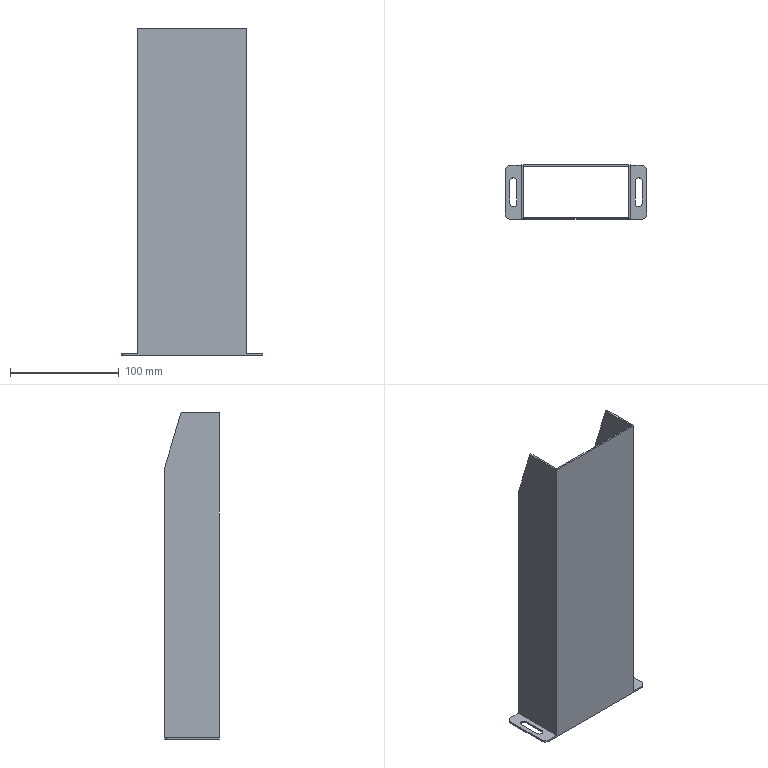Part | SolidWorks | features ICE 4, Cut 1, Fillet 1, MirrorPattern 1, Shell 1 | 1 solid | 29 faces | box 130 x 50 x 300 mm | volume 125628 mm3 | plane 21 | cylinder 8 | commonest cylinder face diameters 6.5 x4 10 x4
STEP:
#1=CARTESIAN_POINT('',(48.5,25.,250.));
#2=VERTEX_POINT('',#1);
#3=CARTESIAN_POINT('',(50.,25.,250.));
#4=VERTEX_POINT('',#3);
#5=CARTESIAN_POINT('',(-65.,25.,250.));
#6=DIRECTION('',(1.,0.,0.));
#7=VECTOR('',#6,1000.);
#8=LINE('',#5,#7);
#9=EDGE_CURVE('',#2,#4,#8,.T.);
#10=ORIENTED_EDGE('',*,*,#9,.F.);
#11=CARTESIAN_POINT('',(48.5,10.,300.));
#12=VERTEX_POINT('',#11);
#13=CARTESIAN_POINT('',(48.5,11.239,295.872));
#14=DIRECTION('',(0.,-0.2873,0.9578));
#15=VECTOR('',#14,1000.);
#16=LINE('',#13,#15);
#17=EDGE_CURVE('',#2,#12,#16,.T.);
#18=ORIENTED_EDGE('',*,*,#17,.T.);
#19=CARTESIAN_POINT('',(50.,10.,300.));
#20=VERTEX_POINT('',#19);
#21=CARTESIAN_POINT('',(-65.,10.,300.));
#22=DIRECTION('',(1.,0.,0.));
#23=VECTOR('',#22,1000.);
#24=LINE('',#21,#23);
#25=EDGE_CURVE('',#12,#20,#24,.T.);
#26=ORIENTED_EDGE('',*,*,#25,.T.);
#27=CARTESIAN_POINT('',(50.,10.,300.));
#28=DIRECTION('',(0.,0.2873,-0.9578));
#29=VECTOR('',#28,1000.);
#30=LINE('',#27,#29);
#31=EDGE_CURVE('',#20,#4,#30,.T.);
#32=ORIENTED_EDGE('',*,*,#31,.T.);
#33=EDGE_LOOP('',(#10,#18,#26,#32));
#34=FACE_OUTER_BOUND('',#33,.T.);
#35=CARTESIAN_POINT('',(-65.,10.,300.));
#36=DIRECTION('',(0.,-0.9578,-0.2873));
#37=DIRECTION('',(0.,0.2873,-0.9578));
#38=AXIS2_PLACEMENT_3D('',#35,#36,#37);
#39=PLANE('',#38);
#40=ADVANCED_FACE('',(#34),#39,.F.);
#41=CARTESIAN_POINT('',(65.,20.,0.));
#42=VERTEX_POINT('',#41);
#43=CARTESIAN_POINT('',(65.,-20.,0.));
#44=VERTEX_POINT('',#43);
#45=CARTESIAN_POINT('',(65.,-25.,0.));
#46=DIRECTION('',(0.,-1.,0.));
#47=VECTOR('',#46,1000.);
#48=LINE('',#45,#47);
#49=EDGE_CURVE('',#42,#44,#48,.T.);
#50=ORIENTED_EDGE('',*,*,#49,.T.);
#51=CARTESIAN_POINT('',(60.,-25.,0.));
#52=VERTEX_POINT('',#51);
#53=CARTESIAN_POINT('',(60.,-20.,0.));
#54=DIRECTION('',(0.,0.,-1.));
#55=DIRECTION('',(1.,0.,0.));
#56=AXIS2_PLACEMENT_3D('',#53,#54,#55);
#57=CIRCLE('',#56,5.);
#58=EDGE_CURVE('',#44,#52,#57,.T.);
#59=ORIENTED_EDGE('',*,*,#58,.T.);
#60=CARTESIAN_POINT('',(-60.,-25.,0.));
#61=VERTEX_POINT('',#60);
#62=CARTESIAN_POINT('',(-50.,-25.,0.));
#63=DIRECTION('',(1.,0.,0.));
#64=VECTOR('',#63,1000.);
#65=LINE('',#62,#64);
#66=EDGE_CURVE('',#61,#52,#65,.T.);
#67=ORIENTED_EDGE('',*,*,#66,.F.);
#68=CARTESIAN_POINT('',(-65.,-20.,0.));
#69=VERTEX_POINT('',#68);
#70=CARTESIAN_POINT('',(-60.,-20.,0.));
#71=DIRECTION('',(0.,0.,-1.));
#72=DIRECTION('',(1.,0.,0.));
#73=AXIS2_PLACEMENT_3D('',#70,#71,#72);
#74=CIRCLE('',#73,5.);
#75=EDGE_CURVE('',#61,#69,#74,.T.);
#76=ORIENTED_EDGE('',*,*,#75,.T.);
#77=CARTESIAN_POINT('',(-65.,20.,0.));
#78=VERTEX_POINT('',#77);
#79=CARTESIAN_POINT('',(-65.,-25.,0.));
#80=DIRECTION('',(0.,1.,0.));
#81=VECTOR('',#80,1000.);
#82=LINE('',#79,#81);
#83=EDGE_CURVE('',#69,#78,#82,.T.);
#84=ORIENTED_EDGE('',*,*,#83,.T.);
#85=CARTESIAN_POINT('',(-60.,25.,0.));
#86=VERTEX_POINT('',#85);
#87=CARTESIAN_POINT('',(-60.,20.,0.));
#88=DIRECTION('',(0.,0.,-1.));
#89=DIRECTION('',(1.,0.,0.));
#90=AXIS2_PLACEMENT_3D('',#87,#88,#89);
#91=CIRCLE('',#90,5.);
#92=EDGE_CURVE('',#78,#86,#91,.T.);
#93=ORIENTED_EDGE('',*,*,#92,.T.);
#94=CARTESIAN_POINT('',(60.,25.,0.));
#95=VERTEX_POINT('',#94);
#96=CARTESIAN_POINT('',(-50.,25.,0.));
#97=DIRECTION('',(-1.,0.,0.));
#98=VECTOR('',#97,1000.);
#99=LINE('',#96,#98);
#100=EDGE_CURVE('',#95,#86,#99,.T.);
#101=ORIENTED_EDGE('',*,*,#100,.F.);
#102=CARTESIAN_POINT('',(60.,20.,0.));
#103=DIRECTION('',(0.,0.,-1.));
#104=DIRECTION('',(1.,0.,0.));
#105=AXIS2_PLACEMENT_3D('',#102,#103,#104);
#106=CIRCLE('',#105,5.);
#107=EDGE_CURVE('',#95,#42,#106,.T.);
#108=ORIENTED_EDGE('',*,*,#107,.T.);
#109=EDGE_LOOP('',(#50,#59,#67,#76,#84,#93,#101,#108));
#110=FACE_OUTER_BOUND('',#109,.T.);
#111=CARTESIAN_POINT('',(-48.5,-23.5,0.));
#112=VERTEX_POINT('',#111);
#113=CARTESIAN_POINT('',(48.5,-23.5,0.));
#114=VERTEX_POINT('',#113);
#115=CARTESIAN_POINT('',(-50.,-23.5,0.));
#116=DIRECTION('',(1.,0.,0.));
#117=VECTOR('',#116,1000.);
#118=LINE('',#115,#117);
#119=EDGE_CURVE('',#112,#114,#118,.T.);
#120=ORIENTED_EDGE('',*,*,#119,.T.);
#121=CARTESIAN_POINT('',(48.5,23.5,0.));
#122=VERTEX_POINT('',#121);
#123=CARTESIAN_POINT('',(48.5,25.,0.));
#124=DIRECTION('',(0.,1.,0.));
#125=VECTOR('',#124,1000.);
#126=LINE('',#123,#125);
#127=EDGE_CURVE('',#114,#122,#126,.T.);
#128=ORIENTED_EDGE('',*,*,#127,.T.);
#129=CARTESIAN_POINT('',(-48.5,23.5,0.));
#130=VERTEX_POINT('',#129);
#131=CARTESIAN_POINT('',(-50.,23.5,0.));
#132=DIRECTION('',(-1.,0.,0.));
#133=VECTOR('',#132,1000.);
#134=LINE('',#131,#133);
#135=EDGE_CURVE('',#122,#130,#134,.T.);
#136=ORIENTED_EDGE('',*,*,#135,.T.);
#137=CARTESIAN_POINT('',(-48.5,25.,0.));
#138=DIRECTION('',(0.,-1.,0.));
#139=VECTOR('',#138,1000.);
#140=LINE('',#137,#139);
#141=EDGE_CURVE('',#130,#112,#140,.T.);
#142=ORIENTED_EDGE('',*,*,#141,.T.);
#143=EDGE_LOOP('',(#120,#128,#136,#142));
#144=FACE_BOUND('',#143,.T.);
#145=CARTESIAN_POINT('',(-60.75,10.,0.));
#146=VERTEX_POINT('',#145);
#147=CARTESIAN_POINT('',(-60.75,-10.,0.));
#148=VERTEX_POINT('',#147);
#149=CARTESIAN_POINT('',(-60.75,-10.,0.));
#150=DIRECTION('',(0.,-1.,0.));
#151=VECTOR('',#150,1000.);
#152=LINE('',#149,#151);
#153=EDGE_CURVE('',#146,#148,#152,.T.);
#154=ORIENTED_EDGE('',*,*,#153,.T.);
#155=CARTESIAN_POINT('',(-54.25,-10.,0.));
#156=VERTEX_POINT('',#155);
#157=CARTESIAN_POINT('',(-57.5,-10.,0.));
#158=DIRECTION('',(0.,0.,1.));
#159=DIRECTION('',(1.,0.,0.));
#160=AXIS2_PLACEMENT_3D('',#157,#158,#159);
#161=CIRCLE('',#160,3.25);
#162=EDGE_CURVE('',#148,#156,#161,.T.);
#163=ORIENTED_EDGE('',*,*,#162,.T.);
#164=CARTESIAN_POINT('',(-54.25,10.,0.));
#165=VERTEX_POINT('',#164);
#166=CARTESIAN_POINT('',(-54.25,-10.,0.));
#167=DIRECTION('',(0.,1.,0.));
#168=VECTOR('',#167,1000.);
#169=LINE('',#166,#168);
#170=EDGE_CURVE('',#156,#165,#169,.T.);
#171=ORIENTED_EDGE('',*,*,#170,.T.);
#172=CARTESIAN_POINT('',(-57.5,10.,0.));
#173=DIRECTION('',(0.,0.,1.));
#174=DIRECTION('',(1.,0.,0.));
#175=AXIS2_PLACEMENT_3D('',#172,#173,#174);
#176=CIRCLE('',#175,3.25);
#177=EDGE_CURVE('',#165,#146,#176,.T.);
#178=ORIENTED_EDGE('',*,*,#177,.T.);
#179=EDGE_LOOP('',(#154,#163,#171,#178));
#180=FACE_BOUND('',#179,.T.);
#181=CARTESIAN_POINT('',(60.75,-10.,0.));
#182=VERTEX_POINT('',#181);
#183=CARTESIAN_POINT('',(54.25,-10.,0.));
#184=VERTEX_POINT('',#183);
#185=CARTESIAN_POINT('',(57.5,-10.,0.));
#186=DIRECTION('',(0.,0.,-1.));
#187=DIRECTION('',(-1.,0.,0.));
#188=AXIS2_PLACEMENT_3D('',#185,#186,#187);
#189=CIRCLE('',#188,3.25);
#190=EDGE_CURVE('',#182,#184,#189,.T.);
#191=ORIENTED_EDGE('',*,*,#190,.F.);
#192=CARTESIAN_POINT('',(60.75,10.,0.));
#193=VERTEX_POINT('',#192);
#194=CARTESIAN_POINT('',(60.75,-10.,0.));
#195=DIRECTION('',(0.,-1.,0.));
#196=VECTOR('',#195,1000.);
#197=LINE('',#194,#196);
#198=EDGE_CURVE('',#193,#182,#197,.T.);
#199=ORIENTED_EDGE('',*,*,#198,.F.);
#200=CARTESIAN_POINT('',(54.25,10.,0.));
#201=VERTEX_POINT('',#200);
#202=CARTESIAN_POINT('',(57.5,10.,0.));
#203=DIRECTION('',(0.,0.,-1.));
#204=DIRECTION('',(-1.,0.,0.));
#205=AXIS2_PLACEMENT_3D('',#202,#203,#204);
#206=CIRCLE('',#205,3.25);
#207=EDGE_CURVE('',#201,#193,#206,.T.);
#208=ORIENTED_EDGE('',*,*,#207,.F.);
#209=CARTESIAN_POINT('',(54.25,-10.,0.));
#210=DIRECTION('',(0.,1.,0.));
#211=VECTOR('',#210,1000.);
#212=LINE('',#209,#211);
#213=EDGE_CURVE('',#184,#201,#212,.T.);
#214=ORIENTED_EDGE('',*,*,#213,.F.);
#215=EDGE_LOOP('',(#191,#199,#208,#214));
#216=FACE_BOUND('',#215,.T.);
#217=CARTESIAN_POINT('',(0.,0.,0.));
#218=DIRECTION('',(0.,0.,1.));
#219=DIRECTION('',(1.,0.,0.));
#220=AXIS2_PLACEMENT_3D('',#217,#218,#219);
#221=PLANE('',#220);
#222=ADVANCED_FACE('',(#110,#144,#180,#216),#221,.F.);
#223=CARTESIAN_POINT('',(60.,-25.,1.5));
#224=VERTEX_POINT('',#223);
#225=CARTESIAN_POINT('',(50.,-25.,1.5));
#226=VERTEX_POINT('',#225);
#227=CARTESIAN_POINT('',(50.,-25.,1.5));
#228=DIRECTION('',(-1.,0.,0.));
#229=VECTOR('',#228,1000.);
#230=LINE('',#227,#229);
#231=EDGE_CURVE('',#224,#226,#230,.T.);
#232=ORIENTED_EDGE('',*,*,#231,.F.);
#233=CARTESIAN_POINT('',(65.,-20.,1.5));
#234=VERTEX_POINT('',#233);
#235=CARTESIAN_POINT('',(60.,-20.,1.5));
#236=DIRECTION('',(0.,0.,1.));
#237=DIRECTION('',(-1.,0.,0.));
#238=AXIS2_PLACEMENT_3D('',#235,#236,#237);
#239=CIRCLE('',#238,5.);
#240=EDGE_CURVE('',#224,#234,#239,.T.);
#241=ORIENTED_EDGE('',*,*,#240,.T.);
#242=CARTESIAN_POINT('',(65.,20.,1.5));
#243=VERTEX_POINT('',#242);
#244=CARTESIAN_POINT('',(65.,-25.,1.5));
#245=DIRECTION('',(0.,-1.,0.));
#246=VECTOR('',#245,1000.);
#247=LINE('',#244,#246);
#248=EDGE_CURVE('',#243,#234,#247,.T.);
#249=ORIENTED_EDGE('',*,*,#248,.F.);
#250=CARTESIAN_POINT('',(60.,25.,1.5));
#251=VERTEX_POINT('',#250);
#252=CARTESIAN_POINT('',(60.,20.,1.5));
#253=DIRECTION('',(0.,0.,1.));
#254=DIRECTION('',(-1.,0.,0.));
#255=AXIS2_PLACEMENT_3D('',#252,#253,#254);
#256=CIRCLE('',#255,5.);
#257=EDGE_CURVE('',#243,#251,#256,.T.);
#258=ORIENTED_EDGE('',*,*,#257,.T.);
#259=CARTESIAN_POINT('',(50.,25.,1.5));
#260=VERTEX_POINT('',#259);
#261=CARTESIAN_POINT('',(50.,25.,1.5));
#262=DIRECTION('',(1.,0.,0.));
#263=VECTOR('',#262,1000.);
#264=LINE('',#261,#263);
#265=EDGE_CURVE('',#260,#251,#264,.T.);
#266=ORIENTED_EDGE('',*,*,#265,.F.);
#267=CARTESIAN_POINT('',(50.,-25.,1.5));
#268=DIRECTION('',(0.,1.,0.));
#269=VECTOR('',#268,1000.);
#270=LINE('',#267,#269);
#271=EDGE_CURVE('',#226,#260,#270,.T.);
#272=ORIENTED_EDGE('',*,*,#271,.F.);
#273=EDGE_LOOP('',(#232,#241,#249,#258,#266,#272));
#274=FACE_OUTER_BOUND('',#273,.T.);
#275=CARTESIAN_POINT('',(60.75,-10.,1.5));
#276=VERTEX_POINT('',#275);
#277=CARTESIAN_POINT('',(54.25,-10.,1.5));
#278=VERTEX_POINT('',#277);
#279=CARTESIAN_POINT('',(57.5,-10.,1.5));
#280=DIRECTION('',(0.,0.,-1.));
#281=DIRECTION('',(-1.,0.,0.));
#282=AXIS2_PLACEMENT_3D('',#279,#280,#281);
#283=CIRCLE('',#282,3.25);
#284=EDGE_CURVE('',#276,#278,#283,.T.);
#285=ORIENTED_EDGE('',*,*,#284,.T.);
#286=CARTESIAN_POINT('',(54.25,10.,1.5));
#287=VERTEX_POINT('',#286);
#288=CARTESIAN_POINT('',(54.25,-10.,1.5));
#289=DIRECTION('',(0.,1.,0.));
#290=VECTOR('',#289,1000.);
#291=LINE('',#288,#290);
#292=EDGE_CURVE('',#278,#287,#291,.T.);
#293=ORIENTED_EDGE('',*,*,#292,.T.);
#294=CARTESIAN_POINT('',(60.75,10.,1.5));
#295=VERTEX_POINT('',#294);
#296=CARTESIAN_POINT('',(57.5,10.,1.5));
#297=DIRECTION('',(0.,0.,-1.));
#298=DIRECTION('',(-1.,0.,0.));
#299=AXIS2_PLACEMENT_3D('',#296,#297,#298);
#300=CIRCLE('',#299,3.25);
#301=EDGE_CURVE('',#287,#295,#300,.T.);
#302=ORIENTED_EDGE('',*,*,#301,.T.);
#303=CARTESIAN_POINT('',(60.75,-10.,1.5));
#304=DIRECTION('',(0.,-1.,0.));
#305=VECTOR('',#304,1000.);
#306=LINE('',#303,#305);
#307=EDGE_CURVE('',#295,#276,#306,.T.);
#308=ORIENTED_EDGE('',*,*,#307,.T.);
#309=EDGE_LOOP('',(#285,#293,#302,#308));
#310=FACE_BOUND('',#309,.T.);
#311=CARTESIAN_POINT('',(0.,0.,1.5));
#312=DIRECTION('',(0.,0.,-1.));
#313=DIRECTION('',(-1.,0.,0.));
#314=AXIS2_PLACEMENT_3D('',#311,#312,#313);
#315=PLANE('',#314);
#316=ADVANCED_FACE('',(#274,#310),#315,.F.);
#317=CARTESIAN_POINT('',(50.,25.,300.));
#318=DIRECTION('',(0.,0.,-1.));
#319=VECTOR('',#318,1000.);
#320=LINE('',#317,#319);
#321=EDGE_CURVE('',#4,#260,#320,.T.);
#322=ORIENTED_EDGE('',*,*,#321,.F.);
#323=ORIENTED_EDGE('',*,*,#31,.F.);
#324=CARTESIAN_POINT('',(50.,-25.,300.));
#325=VERTEX_POINT('',#324);
#326=CARTESIAN_POINT('',(50.,25.,300.));
#327=DIRECTION('',(0.,1.,0.));
#328=VECTOR('',#327,1000.);
#329=LINE('',#326,#328);
#330=EDGE_CURVE('',#325,#20,#329,.T.);
#331=ORIENTED_EDGE('',*,*,#330,.F.);
#332=CARTESIAN_POINT('',(50.,-25.,300.));
#333=DIRECTION('',(0.,0.,-1.));
#334=VECTOR('',#333,1000.);
#335=LINE('',#332,#334);
#336=EDGE_CURVE('',#325,#226,#335,.T.);
#337=ORIENTED_EDGE('',*,*,#336,.T.);
#338=ORIENTED_EDGE('',*,*,#271,.T.);
#339=EDGE_LOOP('',(#322,#323,#331,#337,#338));
#340=FACE_OUTER_BOUND('',#339,.T.);
#341=CARTESIAN_POINT('',(50.,25.,300.));
#342=DIRECTION('',(-1.,0.,0.));
#343=DIRECTION('',(0.,-1.,0.));
#344=AXIS2_PLACEMENT_3D('',#341,#342,#343);
#345=PLANE('',#344);
#346=ADVANCED_FACE('',(#340),#345,.F.);
#347=ORIENTED_EDGE('',*,*,#265,.T.);
#348=CARTESIAN_POINT('',(60.,25.,0.));
#349=DIRECTION('',(0.,0.,-1.));
#350=VECTOR('',#349,1000.);
#351=LINE('',#348,#350);
#352=EDGE_CURVE('',#251,#95,#351,.T.);
#353=ORIENTED_EDGE('',*,*,#352,.T.);
#354=ORIENTED_EDGE('',*,*,#100,.T.);
#355=CARTESIAN_POINT('',(-60.,25.,1.5));
#356=VERTEX_POINT('',#355);
#357=CARTESIAN_POINT('',(-60.,25.,1.5));
#358=DIRECTION('',(0.,0.,1.));
#359=VECTOR('',#358,1000.);
#360=LINE('',#357,#359);
#361=EDGE_CURVE('',#86,#356,#360,.T.);
#362=ORIENTED_EDGE('',*,*,#361,.T.);
#363=CARTESIAN_POINT('',(-50.,25.,1.5));
#364=VERTEX_POINT('',#363);
#365=CARTESIAN_POINT('',(-65.,25.,1.5));
#366=DIRECTION('',(1.,0.,0.));
#367=VECTOR('',#366,1000.);
#368=LINE('',#365,#367);
#369=EDGE_CURVE('',#356,#364,#368,.T.);
#370=ORIENTED_EDGE('',*,*,#369,.T.);
#371=CARTESIAN_POINT('',(-50.,25.,250.));
#372=VERTEX_POINT('',#371);
#373=CARTESIAN_POINT('',(-50.,25.,300.));
#374=DIRECTION('',(0.,0.,-1.));
#375=VECTOR('',#374,1000.);
#376=LINE('',#373,#375);
#377=EDGE_CURVE('',#372,#364,#376,.T.);
#378=ORIENTED_EDGE('',*,*,#377,.F.);
#379=CARTESIAN_POINT('',(-48.5,25.,250.));
#380=VERTEX_POINT('',#379);
#381=CARTESIAN_POINT('',(-65.,25.,250.));
#382=DIRECTION('',(1.,0.,0.));
#383=VECTOR('',#382,1000.);
#384=LINE('',#381,#383);
#385=EDGE_CURVE('',#372,#380,#384,.T.);
#386=ORIENTED_EDGE('',*,*,#385,.T.);
#387=CARTESIAN_POINT('',(-48.5,25.,250.));
#388=DIRECTION('',(-1.,0.,0.));
#389=VECTOR('',#388,1000.);
#390=LINE('',#387,#389);
#391=EDGE_CURVE('',#2,#380,#390,.T.);
#392=ORIENTED_EDGE('',*,*,#391,.F.);
#393=ORIENTED_EDGE('',*,*,#9,.T.);
#394=ORIENTED_EDGE('',*,*,#321,.T.);
#395=EDGE_LOOP('',(#347,#353,#354,#362,#370,#378,#386,#392,#393,#394));
#396=FACE_OUTER_BOUND('',#395,.T.);
#397=CARTESIAN_POINT('',(-50.,25.,300.));
#398=DIRECTION('',(0.,-1.,0.));
#399=DIRECTION('',(0.,0.,-1.));
#400=AXIS2_PLACEMENT_3D('',#397,#398,#399);
#401=PLANE('',#400);
#402=ADVANCED_FACE('',(#396),#401,.F.);
#403=CARTESIAN_POINT('',(-50.,10.,300.));
#404=VERTEX_POINT('',#403);
#405=CARTESIAN_POINT('',(-50.,-25.,300.));
#406=VERTEX_POINT('',#405);
#407=CARTESIAN_POINT('',(-50.,25.,300.));
#408=DIRECTION('',(0.,-1.,0.));
#409=VECTOR('',#408,1000.);
#410=LINE('',#407,#409);
#411=EDGE_CURVE('',#404,#406,#410,.T.);
#412=ORIENTED_EDGE('',*,*,#411,.F.);
#413=CARTESIAN_POINT('',(-50.,11.239,295.872));
#414=DIRECTION('',(0.,0.2873,-0.9578));
#415=VECTOR('',#414,1000.);
#416=LINE('',#413,#415);
#417=EDGE_CURVE('',#404,#372,#416,.T.);
#418=ORIENTED_EDGE('',*,*,#417,.T.);
#419=ORIENTED_EDGE('',*,*,#377,.T.);
#420=CARTESIAN_POINT('',(-50.,-25.,1.5));
#421=VERTEX_POINT('',#420);
#422=CARTESIAN_POINT('',(-50.,-25.,1.5));
#423=DIRECTION('',(0.,-1.,0.));
#424=VECTOR('',#423,1000.);
#425=LINE('',#422,#424);
#426=EDGE_CURVE('',#364,#421,#425,.T.);
#427=ORIENTED_EDGE('',*,*,#426,.T.);
#428=CARTESIAN_POINT('',(-50.,-25.,300.));
#429=DIRECTION('',(0.,0.,-1.));
#430=VECTOR('',#429,1000.);
#431=LINE('',#428,#430);
#432=EDGE_CURVE('',#406,#421,#431,.T.);
#433=ORIENTED_EDGE('',*,*,#432,.F.);
#434=EDGE_LOOP('',(#412,#418,#419,#427,#433));
#435=FACE_OUTER_BOUND('',#434,.T.);
#436=CARTESIAN_POINT('',(-50.,25.,300.));
#437=DIRECTION('',(1.,0.,0.));
#438=DIRECTION('',(0.,1.,0.));
#439=AXIS2_PLACEMENT_3D('',#436,#437,#438);
#440=PLANE('',#439);
#441=ADVANCED_FACE('',(#435),#440,.F.);
#442=ORIENTED_EDGE('',*,*,#66,.T.);
#443=CARTESIAN_POINT('',(60.,-25.,1.5));
#444=DIRECTION('',(0.,0.,1.));
#445=VECTOR('',#444,1000.);
#446=LINE('',#443,#445);
#447=EDGE_CURVE('',#52,#224,#446,.T.);
#448=ORIENTED_EDGE('',*,*,#447,.T.);
#449=ORIENTED_EDGE('',*,*,#231,.T.);
#450=ORIENTED_EDGE('',*,*,#336,.F.);
#451=CARTESIAN_POINT('',(-50.,-25.,300.));
#452=DIRECTION('',(1.,0.,0.));
#453=VECTOR('',#452,1000.);
#454=LINE('',#451,#453);
#455=EDGE_CURVE('',#406,#325,#454,.T.);
#456=ORIENTED_EDGE('',*,*,#455,.F.);
#457=ORIENTED_EDGE('',*,*,#432,.T.);
#458=CARTESIAN_POINT('',(-60.,-25.,1.5));
#459=VERTEX_POINT('',#458);
#460=CARTESIAN_POINT('',(-65.,-25.,1.5));
#461=DIRECTION('',(-1.,0.,0.));
#462=VECTOR('',#461,1000.);
#463=LINE('',#460,#462);
#464=EDGE_CURVE('',#421,#459,#463,.T.);
#465=ORIENTED_EDGE('',*,*,#464,.T.);
#466=CARTESIAN_POINT('',(-60.,-25.,0.));
#467=DIRECTION('',(0.,0.,-1.));
#468=VECTOR('',#467,1000.);
#469=LINE('',#466,#468);
#470=EDGE_CURVE('',#459,#61,#469,.T.);
#471=ORIENTED_EDGE('',*,*,#470,.T.);
#472=EDGE_LOOP('',(#442,#448,#449,#450,#456,#457,#465,#471));
#473=FACE_OUTER_BOUND('',#472,.T.);
#474=CARTESIAN_POINT('',(-50.,-25.,300.));
#475=DIRECTION('',(0.,1.,0.));
#476=DIRECTION('',(0.,0.,1.));
#477=AXIS2_PLACEMENT_3D('',#474,#475,#476);
#478=PLANE('',#477);
#479=ADVANCED_FACE('',(#473),#478,.F.);
#480=CARTESIAN_POINT('',(-48.5,10.,300.));
#481=VERTEX_POINT('',#480);
#482=CARTESIAN_POINT('',(-65.,10.,300.));
#483=DIRECTION('',(1.,0.,0.));
#484=VECTOR('',#483,1000.);
#485=LINE('',#482,#484);
#486=EDGE_CURVE('',#404,#481,#485,.T.);
#487=ORIENTED_EDGE('',*,*,#486,.F.);
#488=ORIENTED_EDGE('',*,*,#411,.T.);
#489=ORIENTED_EDGE('',*,*,#455,.T.);
#490=ORIENTED_EDGE('',*,*,#330,.T.);
#491=ORIENTED_EDGE('',*,*,#25,.F.);
#492=CARTESIAN_POINT('',(48.5,-23.5,300.));
#493=VERTEX_POINT('',#492);
#494=CARTESIAN_POINT('',(48.5,25.,300.));
#495=DIRECTION('',(0.,1.,0.));
#496=VECTOR('',#495,1000.);
#497=LINE('',#494,#496);
#498=EDGE_CURVE('',#493,#12,#497,.T.);
#499=ORIENTED_EDGE('',*,*,#498,.F.);
#500=CARTESIAN_POINT('',(-48.5,-23.5,300.));
#501=VERTEX_POINT('',#500);
#502=CARTESIAN_POINT('',(-50.,-23.5,300.));
#503=DIRECTION('',(1.,0.,0.));
#504=VECTOR('',#503,1000.);
#505=LINE('',#502,#504);
#506=EDGE_CURVE('',#501,#493,#505,.T.);
#507=ORIENTED_EDGE('',*,*,#506,.F.);
#508=CARTESIAN_POINT('',(-48.5,25.,300.));
#509=DIRECTION('',(0.,-1.,0.));
#510=VECTOR('',#509,1000.);
#511=LINE('',#508,#510);
#512=EDGE_CURVE('',#481,#501,#511,.T.);
#513=ORIENTED_EDGE('',*,*,#512,.F.);
#514=EDGE_LOOP('',(#487,#488,#489,#490,#491,#499,#507,#513));
#515=FACE_OUTER_BOUND('',#514,.T.);
#516=CARTESIAN_POINT('',(0.,0.,300.));
#517=DIRECTION('',(0.,0.,1.));
#518=DIRECTION('',(1.,0.,0.));
#519=AXIS2_PLACEMENT_3D('',#516,#517,#518);
#520=PLANE('',#519);
#521=ADVANCED_FACE('',(#515),#520,.T.);
#522=ORIENTED_EDGE('',*,*,#17,.F.);
#523=CARTESIAN_POINT('',(48.5,23.5,250.));
#524=VERTEX_POINT('',#523);
#525=CARTESIAN_POINT('',(48.5,-25.001,250.));
#526=DIRECTION('',(0.,1.,0.));
#527=VECTOR('',#526,1000.);
#528=LINE('',#525,#527);
#529=EDGE_CURVE('',#524,#2,#528,.T.);
#530=ORIENTED_EDGE('',*,*,#529,.F.);
#531=CARTESIAN_POINT('',(48.5,23.5,300.));
#532=DIRECTION('',(0.,0.,-1.));
#533=VECTOR('',#532,1000.);
#534=LINE('',#531,#533);
#535=EDGE_CURVE('',#524,#122,#534,.T.);
#536=ORIENTED_EDGE('',*,*,#535,.T.);
#537=ORIENTED_EDGE('',*,*,#127,.F.);
#538=CARTESIAN_POINT('',(48.5,-23.5,300.));
#539=DIRECTION('',(0.,0.,-1.));
#540=VECTOR('',#539,1000.);
#541=LINE('',#538,#540);
#542=EDGE_CURVE('',#493,#114,#541,.T.);
#543=ORIENTED_EDGE('',*,*,#542,.F.);
#544=ORIENTED_EDGE('',*,*,#498,.T.);
#545=EDGE_LOOP('',(#522,#530,#536,#537,#543,#544));
#546=FACE_OUTER_BOUND('',#545,.T.);
#547=CARTESIAN_POINT('',(48.5,25.,300.));
#548=DIRECTION('',(-1.,0.,0.));
#549=DIRECTION('',(0.,-1.,0.));
#550=AXIS2_PLACEMENT_3D('',#547,#548,#549);
#551=PLANE('',#550);
#552=ADVANCED_FACE('',(#546),#551,.T.);
#553=CARTESIAN_POINT('',(-48.5,23.5,250.));
#554=VERTEX_POINT('',#553);
#555=CARTESIAN_POINT('',(-48.5,23.5,250.));
#556=DIRECTION('',(-1.,0.,0.));
#557=VECTOR('',#556,1000.);
#558=LINE('',#555,#557);
#559=EDGE_CURVE('',#524,#554,#558,.T.);
#560=ORIENTED_EDGE('',*,*,#559,.T.);
#561=CARTESIAN_POINT('',(-48.5,23.5,300.));
#562=DIRECTION('',(0.,0.,-1.));
#563=VECTOR('',#562,1000.);
#564=LINE('',#561,#563);
#565=EDGE_CURVE('',#554,#130,#564,.T.);
#566=ORIENTED_EDGE('',*,*,#565,.T.);
#567=ORIENTED_EDGE('',*,*,#135,.F.);
#568=ORIENTED_EDGE('',*,*,#535,.F.);
#569=EDGE_LOOP('',(#560,#566,#567,#568));
#570=FACE_OUTER_BOUND('',#569,.T.);
#571=CARTESIAN_POINT('',(-50.,23.5,300.));
#572=DIRECTION('',(0.,-1.,0.));
#573=DIRECTION('',(0.,0.,-1.));
#574=AXIS2_PLACEMENT_3D('',#571,#572,#573);
#575=PLANE('',#574);
#576=ADVANCED_FACE('',(#570),#575,.T.);
#577=CARTESIAN_POINT('',(-48.5,11.239,295.872));
#578=DIRECTION('',(0.,0.2873,-0.9578));
#579=VECTOR('',#578,1000.);
#580=LINE('',#577,#579);
#581=EDGE_CURVE('',#481,#380,#580,.T.);
#582=ORIENTED_EDGE('',*,*,#581,.F.);
#583=ORIENTED_EDGE('',*,*,#512,.T.);
#584=CARTESIAN_POINT('',(-48.5,-23.5,300.));
#585=DIRECTION('',(0.,0.,-1.));
#586=VECTOR('',#585,1000.);
#587=LINE('',#584,#586);
#588=EDGE_CURVE('',#501,#112,#587,.T.);
#589=ORIENTED_EDGE('',*,*,#588,.T.);
#590=ORIENTED_EDGE('',*,*,#141,.F.);
#591=ORIENTED_EDGE('',*,*,#565,.F.);
#592=CARTESIAN_POINT('',(-48.5,-25.001,250.));
#593=DIRECTION('',(0.,1.,0.));
#594=VECTOR('',#593,1000.);
#595=LINE('',#592,#594);
#596=EDGE_CURVE('',#554,#380,#595,.T.);
#597=ORIENTED_EDGE('',*,*,#596,.T.);
#598=EDGE_LOOP('',(#582,#583,#589,#590,#591,#597));
#599=FACE_OUTER_BOUND('',#598,.T.);
#600=CARTESIAN_POINT('',(-48.5,25.,300.));
#601=DIRECTION('',(1.,0.,0.));
#602=DIRECTION('',(0.,1.,0.));
#603=AXIS2_PLACEMENT_3D('',#600,#601,#602);
#604=PLANE('',#603);
#605=ADVANCED_FACE('',(#599),#604,.T.);
#606=ORIENTED_EDGE('',*,*,#119,.F.);
#607=ORIENTED_EDGE('',*,*,#588,.F.);
#608=ORIENTED_EDGE('',*,*,#506,.T.);
#609=ORIENTED_EDGE('',*,*,#542,.T.);
#610=EDGE_LOOP('',(#606,#607,#608,#609));
#611=FACE_OUTER_BOUND('',#610,.T.);
#612=CARTESIAN_POINT('',(-50.,-23.5,300.));
#613=DIRECTION('',(0.,1.,0.));
#614=DIRECTION('',(0.,0.,1.));
#615=AXIS2_PLACEMENT_3D('',#612,#613,#614);
#616=PLANE('',#615);
#617=ADVANCED_FACE('',(#611),#616,.T.);
#618=ORIENTED_EDGE('',*,*,#248,.T.);
#619=CARTESIAN_POINT('',(65.,-20.,0.));
#620=DIRECTION('',(0.,0.,-1.));
#621=VECTOR('',#620,1000.);
#622=LINE('',#619,#621);
#623=EDGE_CURVE('',#234,#44,#622,.T.);
#624=ORIENTED_EDGE('',*,*,#623,.T.);
#625=ORIENTED_EDGE('',*,*,#49,.F.);
#626=CARTESIAN_POINT('',(65.,20.,1.5));
#627=DIRECTION('',(0.,0.,1.));
#628=VECTOR('',#627,1000.);
#629=LINE('',#626,#628);
#630=EDGE_CURVE('',#42,#243,#629,.T.);
#631=ORIENTED_EDGE('',*,*,#630,.T.);
#632=EDGE_LOOP('',(#618,#624,#625,#631));
#633=FACE_OUTER_BOUND('',#632,.T.);
#634=CARTESIAN_POINT('',(65.,-25.,1.5));
#635=DIRECTION('',(1.,0.,0.));
#636=DIRECTION('',(0.,0.,-1.));
#637=AXIS2_PLACEMENT_3D('',#634,#635,#636);
#638=PLANE('',#637);
#639=ADVANCED_FACE('',(#633),#638,.T.);
#640=ORIENTED_EDGE('',*,*,#83,.F.);
#641=CARTESIAN_POINT('',(-65.,-20.,1.5));
#642=VERTEX_POINT('',#641);
#643=CARTESIAN_POINT('',(-65.,-20.,1.5));
#644=DIRECTION('',(0.,0.,1.));
#645=VECTOR('',#644,1000.);
#646=LINE('',#643,#645);
#647=EDGE_CURVE('',#69,#642,#646,.T.);
#648=ORIENTED_EDGE('',*,*,#647,.T.);
#649=CARTESIAN_POINT('',(-65.,20.,1.5));
#650=VERTEX_POINT('',#649);
#651=CARTESIAN_POINT('',(-65.,-25.,1.5));
#652=DIRECTION('',(0.,1.,0.));
#653=VECTOR('',#652,1000.);
#654=LINE('',#651,#653);
#655=EDGE_CURVE('',#642,#650,#654,.T.);
#656=ORIENTED_EDGE('',*,*,#655,.T.);
#657=CARTESIAN_POINT('',(-65.,20.,0.));
#658=DIRECTION('',(0.,0.,-1.));
#659=VECTOR('',#658,1000.);
#660=LINE('',#657,#659);
#661=EDGE_CURVE('',#650,#78,#660,.T.);
#662=ORIENTED_EDGE('',*,*,#661,.T.);
#663=EDGE_LOOP('',(#640,#648,#656,#662));
#664=FACE_OUTER_BOUND('',#663,.T.);
#665=CARTESIAN_POINT('',(-65.,-25.,1.5));
#666=DIRECTION('',(-1.,0.,0.));
#667=DIRECTION('',(0.,0.,1.));
#668=AXIS2_PLACEMENT_3D('',#665,#666,#667);
#669=PLANE('',#668);
#670=ADVANCED_FACE('',(#664),#669,.T.);
#671=CARTESIAN_POINT('',(-54.25,-10.,1.5));
#672=VERTEX_POINT('',#671);
#673=CARTESIAN_POINT('',(-54.25,10.,1.5));
#674=VERTEX_POINT('',#673);
#675=CARTESIAN_POINT('',(-54.25,-10.,1.5));
#676=DIRECTION('',(0.,1.,0.));
#677=VECTOR('',#676,1000.);
#678=LINE('',#675,#677);
#679=EDGE_CURVE('',#672,#674,#678,.T.);
#680=ORIENTED_EDGE('',*,*,#679,.F.);
#681=CARTESIAN_POINT('',(-60.75,-10.,1.5));
#682=VERTEX_POINT('',#681);
#683=CARTESIAN_POINT('',(-57.5,-10.,1.5));
#684=DIRECTION('',(0.,0.,1.));
#685=DIRECTION('',(1.,0.,0.));
#686=AXIS2_PLACEMENT_3D('',#683,#684,#685);
#687=CIRCLE('',#686,3.25);
#688=EDGE_CURVE('',#682,#672,#687,.T.);
#689=ORIENTED_EDGE('',*,*,#688,.F.);
#690=CARTESIAN_POINT('',(-60.75,10.,1.5));
#691=VERTEX_POINT('',#690);
#692=CARTESIAN_POINT('',(-60.75,-10.,1.5));
#693=DIRECTION('',(0.,-1.,0.));
#694=VECTOR('',#693,1000.);
#695=LINE('',#692,#694);
#696=EDGE_CURVE('',#691,#682,#695,.T.);
#697=ORIENTED_EDGE('',*,*,#696,.F.);
#698=CARTESIAN_POINT('',(-57.5,10.,1.5));
#699=DIRECTION('',(0.,0.,1.));
#700=DIRECTION('',(1.,0.,0.));
#701=AXIS2_PLACEMENT_3D('',#698,#699,#700);
#702=CIRCLE('',#701,3.25);
#703=EDGE_CURVE('',#674,#691,#702,.T.);
#704=ORIENTED_EDGE('',*,*,#703,.F.);
#705=EDGE_LOOP('',(#680,#689,#697,#704));
#706=FACE_BOUND('',#705,.T.);
#707=ORIENTED_EDGE('',*,*,#655,.F.);
#708=CARTESIAN_POINT('',(-60.,-20.,1.5));
#709=DIRECTION('',(0.,0.,1.));
#710=DIRECTION('',(-1.,0.,0.));
#711=AXIS2_PLACEMENT_3D('',#708,#709,#710);
#712=CIRCLE('',#711,5.);
#713=EDGE_CURVE('',#642,#459,#712,.T.);
#714=ORIENTED_EDGE('',*,*,#713,.T.);
#715=ORIENTED_EDGE('',*,*,#464,.F.);
#716=ORIENTED_EDGE('',*,*,#426,.F.);
#717=ORIENTED_EDGE('',*,*,#369,.F.);
#718=CARTESIAN_POINT('',(-60.,20.,1.5));
#719=DIRECTION('',(0.,0.,1.));
#720=DIRECTION('',(-1.,0.,0.));
#721=AXIS2_PLACEMENT_3D('',#718,#719,#720);
#722=CIRCLE('',#721,5.);
#723=EDGE_CURVE('',#356,#650,#722,.T.);
#724=ORIENTED_EDGE('',*,*,#723,.T.);
#725=EDGE_LOOP('',(#707,#714,#715,#716,#717,#724));
#726=FACE_OUTER_BOUND('',#725,.T.);
#727=CARTESIAN_POINT('',(0.,0.,1.5));
#728=DIRECTION('',(0.,0.,-1.));
#729=DIRECTION('',(-1.,0.,0.));
#730=AXIS2_PLACEMENT_3D('',#727,#728,#729);
#731=PLANE('',#730);
#732=ADVANCED_FACE('',(#706,#726),#731,.F.);
#733=ORIENTED_EDGE('',*,*,#581,.T.);
#734=ORIENTED_EDGE('',*,*,#385,.F.);
#735=ORIENTED_EDGE('',*,*,#417,.F.);
#736=ORIENTED_EDGE('',*,*,#486,.T.);
#737=EDGE_LOOP('',(#733,#734,#735,#736));
#738=FACE_OUTER_BOUND('',#737,.T.);
#739=CARTESIAN_POINT('',(-65.,10.,300.));
#740=DIRECTION('',(0.,-0.9578,-0.2873));
#741=DIRECTION('',(0.,0.2873,-0.9578));
#742=AXIS2_PLACEMENT_3D('',#739,#740,#741);
#743=PLANE('',#742);
#744=ADVANCED_FACE('',(#738),#743,.F.);
#745=ORIENTED_EDGE('',*,*,#240,.F.);
#746=ORIENTED_EDGE('',*,*,#447,.F.);
#747=ORIENTED_EDGE('',*,*,#58,.F.);
#748=ORIENTED_EDGE('',*,*,#623,.F.);
#749=EDGE_LOOP('',(#745,#746,#747,#748));
#750=FACE_OUTER_BOUND('',#749,.T.);
#751=CARTESIAN_POINT('',(60.,-20.,1.5));
#752=DIRECTION('',(0.,0.,1.));
#753=DIRECTION('',(1.,0.,0.));
#754=AXIS2_PLACEMENT_3D('',#751,#752,#753);
#755=CYLINDRICAL_SURFACE('',#754,5.);
#756=ADVANCED_FACE('',(#750),#755,.T.);
#757=ORIENTED_EDGE('',*,*,#257,.F.);
#758=ORIENTED_EDGE('',*,*,#630,.F.);
#759=ORIENTED_EDGE('',*,*,#107,.F.);
#760=ORIENTED_EDGE('',*,*,#352,.F.);
#761=EDGE_LOOP('',(#757,#758,#759,#760));
#762=FACE_OUTER_BOUND('',#761,.T.);
#763=CARTESIAN_POINT('',(60.,20.,300.));
#764=DIRECTION('',(0.,0.,1.));
#765=DIRECTION('',(1.,0.,0.));
#766=AXIS2_PLACEMENT_3D('',#763,#764,#765);
#767=CYLINDRICAL_SURFACE('',#766,5.);
#768=ADVANCED_FACE('',(#762),#767,.T.);
#769=ORIENTED_EDGE('',*,*,#713,.F.);
#770=ORIENTED_EDGE('',*,*,#647,.F.);
#771=ORIENTED_EDGE('',*,*,#75,.F.);
#772=ORIENTED_EDGE('',*,*,#470,.F.);
#773=EDGE_LOOP('',(#769,#770,#771,#772));
#774=FACE_OUTER_BOUND('',#773,.T.);
#775=CARTESIAN_POINT('',(-60.,-20.,300.));
#776=DIRECTION('',(0.,0.,1.));
#777=DIRECTION('',(1.,0.,0.));
#778=AXIS2_PLACEMENT_3D('',#775,#776,#777);
#779=CYLINDRICAL_SURFACE('',#778,5.);
#780=ADVANCED_FACE('',(#774),#779,.T.);
#781=ORIENTED_EDGE('',*,*,#723,.F.);
#782=ORIENTED_EDGE('',*,*,#361,.F.);
#783=ORIENTED_EDGE('',*,*,#92,.F.);
#784=ORIENTED_EDGE('',*,*,#661,.F.);
#785=EDGE_LOOP('',(#781,#782,#783,#784));
#786=FACE_OUTER_BOUND('',#785,.T.);
#787=CARTESIAN_POINT('',(-60.,20.,1.5));
#788=DIRECTION('',(0.,0.,1.));
#789=DIRECTION('',(1.,0.,0.));
#790=AXIS2_PLACEMENT_3D('',#787,#788,#789);
#791=CYLINDRICAL_SURFACE('',#790,5.);
#792=ADVANCED_FACE('',(#786),#791,.T.);
#793=ORIENTED_EDGE('',*,*,#688,.T.);
#794=CARTESIAN_POINT('',(-54.25,-10.,0.));
#795=DIRECTION('',(0.,0.,1.));
#796=VECTOR('',#795,1000.);
#797=LINE('',#794,#796);
#798=EDGE_CURVE('',#156,#672,#797,.T.);
#799=ORIENTED_EDGE('',*,*,#798,.F.);
#800=ORIENTED_EDGE('',*,*,#162,.F.);
#801=CARTESIAN_POINT('',(-60.75,-10.,0.));
#802=DIRECTION('',(0.,0.,1.));
#803=VECTOR('',#802,1000.);
#804=LINE('',#801,#803);
#805=EDGE_CURVE('',#148,#682,#804,.T.);
#806=ORIENTED_EDGE('',*,*,#805,.T.);
#807=EDGE_LOOP('',(#793,#799,#800,#806));
#808=FACE_OUTER_BOUND('',#807,.T.);
#809=CARTESIAN_POINT('',(-57.5,-10.,0.));
#810=DIRECTION('',(0.,0.,1.));
#811=DIRECTION('',(1.,0.,0.));
#812=AXIS2_PLACEMENT_3D('',#809,#810,#811);
#813=CYLINDRICAL_SURFACE('',#812,3.25);
#814=ADVANCED_FACE('',(#808),#813,.F.);
#815=ORIENTED_EDGE('',*,*,#696,.T.);
#816=ORIENTED_EDGE('',*,*,#805,.F.);
#817=ORIENTED_EDGE('',*,*,#153,.F.);
#818=CARTESIAN_POINT('',(-60.75,10.,0.));
#819=DIRECTION('',(0.,0.,1.));
#820=VECTOR('',#819,1000.);
#821=LINE('',#818,#820);
#822=EDGE_CURVE('',#146,#691,#821,.T.);
#823=ORIENTED_EDGE('',*,*,#822,.T.);
#824=EDGE_LOOP('',(#815,#816,#817,#823));
#825=FACE_OUTER_BOUND('',#824,.T.);
#826=CARTESIAN_POINT('',(-60.75,-10.,0.));
#827=DIRECTION('',(-1.,0.,0.));
#828=DIRECTION('',(0.,-1.,0.));
#829=AXIS2_PLACEMENT_3D('',#826,#827,#828);
#830=PLANE('',#829);
#831=ADVANCED_FACE('',(#825),#830,.F.);
#832=ORIENTED_EDGE('',*,*,#703,.T.);
#833=ORIENTED_EDGE('',*,*,#822,.F.);
#834=ORIENTED_EDGE('',*,*,#177,.F.);
#835=CARTESIAN_POINT('',(-54.25,10.,0.));
#836=DIRECTION('',(0.,0.,1.));
#837=VECTOR('',#836,1000.);
#838=LINE('',#835,#837);
#839=EDGE_CURVE('',#165,#674,#838,.T.);
#840=ORIENTED_EDGE('',*,*,#839,.T.);
#841=EDGE_LOOP('',(#832,#833,#834,#840));
#842=FACE_OUTER_BOUND('',#841,.T.);
#843=CARTESIAN_POINT('',(-57.5,10.,0.));
#844=DIRECTION('',(0.,0.,1.));
#845=DIRECTION('',(1.,0.,0.));
#846=AXIS2_PLACEMENT_3D('',#843,#844,#845);
#847=CYLINDRICAL_SURFACE('',#846,3.25);
#848=ADVANCED_FACE('',(#842),#847,.F.);
#849=ORIENTED_EDGE('',*,*,#679,.T.);
#850=ORIENTED_EDGE('',*,*,#839,.F.);
#851=ORIENTED_EDGE('',*,*,#170,.F.);
#852=ORIENTED_EDGE('',*,*,#798,.T.);
#853=EDGE_LOOP('',(#849,#850,#851,#852));
#854=FACE_OUTER_BOUND('',#853,.T.);
#855=CARTESIAN_POINT('',(-54.25,-10.,0.));
#856=DIRECTION('',(1.,0.,0.));
#857=DIRECTION('',(0.,1.,0.));
#858=AXIS2_PLACEMENT_3D('',#855,#856,#857);
#859=PLANE('',#858);
#860=ADVANCED_FACE('',(#854),#859,.F.);
#861=ORIENTED_EDGE('',*,*,#284,.F.);
#862=CARTESIAN_POINT('',(60.75,-10.,0.));
#863=DIRECTION('',(0.,0.,1.));
#864=VECTOR('',#863,1000.);
#865=LINE('',#862,#864);
#866=EDGE_CURVE('',#182,#276,#865,.T.);
#867=ORIENTED_EDGE('',*,*,#866,.F.);
#868=ORIENTED_EDGE('',*,*,#190,.T.);
#869=CARTESIAN_POINT('',(54.25,-10.,0.));
#870=DIRECTION('',(0.,0.,1.));
#871=VECTOR('',#870,1000.);
#872=LINE('',#869,#871);
#873=EDGE_CURVE('',#184,#278,#872,.T.);
#874=ORIENTED_EDGE('',*,*,#873,.T.);
#875=EDGE_LOOP('',(#861,#867,#868,#874));
#876=FACE_OUTER_BOUND('',#875,.T.);
#877=CARTESIAN_POINT('',(57.5,-10.,0.));
#878=DIRECTION('',(0.,0.,1.));
#879=DIRECTION('',(1.,0.,0.));
#880=AXIS2_PLACEMENT_3D('',#877,#878,#879);
#881=CYLINDRICAL_SURFACE('',#880,3.25);
#882=ADVANCED_FACE('',(#876),#881,.F.);
#883=ORIENTED_EDGE('',*,*,#292,.F.);
#884=ORIENTED_EDGE('',*,*,#873,.F.);
#885=ORIENTED_EDGE('',*,*,#213,.T.);
#886=CARTESIAN_POINT('',(54.25,10.,0.));
#887=DIRECTION('',(0.,0.,1.));
#888=VECTOR('',#887,1000.);
#889=LINE('',#886,#888);
#890=EDGE_CURVE('',#201,#287,#889,.T.);
#891=ORIENTED_EDGE('',*,*,#890,.T.);
#892=EDGE_LOOP('',(#883,#884,#885,#891));
#893=FACE_OUTER_BOUND('',#892,.T.);
#894=CARTESIAN_POINT('',(54.25,-10.,0.));
#895=DIRECTION('',(1.,0.,0.));
#896=DIRECTION('',(0.,1.,0.));
#897=AXIS2_PLACEMENT_3D('',#894,#895,#896);
#898=PLANE('',#897);
#899=ADVANCED_FACE('',(#893),#898,.T.);
#900=ORIENTED_EDGE('',*,*,#301,.F.);
#901=ORIENTED_EDGE('',*,*,#890,.F.);
#902=ORIENTED_EDGE('',*,*,#207,.T.);
#903=CARTESIAN_POINT('',(60.75,10.,0.));
#904=DIRECTION('',(0.,0.,1.));
#905=VECTOR('',#904,1000.);
#906=LINE('',#903,#905);
#907=EDGE_CURVE('',#193,#295,#906,.T.);
#908=ORIENTED_EDGE('',*,*,#907,.T.);
#909=EDGE_LOOP('',(#900,#901,#902,#908));
#910=FACE_OUTER_BOUND('',#909,.T.);
#911=CARTESIAN_POINT('',(57.5,10.,0.));
#912=DIRECTION('',(0.,0.,1.));
#913=DIRECTION('',(1.,0.,0.));
#914=AXIS2_PLACEMENT_3D('',#911,#912,#913);
#915=CYLINDRICAL_SURFACE('',#914,3.25);
#916=ADVANCED_FACE('',(#910),#915,.F.);
#917=ORIENTED_EDGE('',*,*,#307,.F.);
#918=ORIENTED_EDGE('',*,*,#907,.F.);
#919=ORIENTED_EDGE('',*,*,#198,.T.);
#920=ORIENTED_EDGE('',*,*,#866,.T.);
#921=EDGE_LOOP('',(#917,#918,#919,#920));
#922=FACE_OUTER_BOUND('',#921,.T.);
#923=CARTESIAN_POINT('',(60.75,-10.,0.));
#924=DIRECTION('',(-1.,0.,0.));
#925=DIRECTION('',(0.,-1.,0.));
#926=AXIS2_PLACEMENT_3D('',#923,#924,#925);
#927=PLANE('',#926);
#928=ADVANCED_FACE('',(#922),#927,.T.);
#929=ORIENTED_EDGE('',*,*,#529,.T.);
#930=ORIENTED_EDGE('',*,*,#391,.T.);
#931=ORIENTED_EDGE('',*,*,#596,.F.);
#932=ORIENTED_EDGE('',*,*,#559,.F.);
#933=EDGE_LOOP('',(#929,#930,#931,#932));
#934=FACE_OUTER_BOUND('',#933,.T.);
#935=CARTESIAN_POINT('',(-48.5,-25.001,250.));
#936=DIRECTION('',(0.,0.,-1.));
#937=DIRECTION('',(-1.,0.,0.));
#938=AXIS2_PLACEMENT_3D('',#935,#936,#937);
#939=PLANE('',#938);
#940=ADVANCED_FACE('',(#934),#939,.F.);
#941=CLOSED_SHELL('',(#40,#222,#316,#346,#402,#441,#479,#521,#552,#576,#605,#617,#639,#670,#732,#744,#756,#768,#780,#792,#814,#831,#848,#860,#882,#899,#916,#928,#940));
#942=MANIFOLD_SOLID_BREP('',#941);
#943=CARTESIAN_POINT('',(0.,0.,0.));
#944=DIRECTION('',(0.,0.,1.));
#945=DIRECTION('',(1.,0.,0.));
#946=AXIS2_PLACEMENT_3D('',#943,#944,#945);
#947=(LENGTH_UNIT()NAMED_UNIT(*)SI_UNIT(.MILLI.,.METRE.));
#948=UNCERTAINTY_MEASURE_WITH_UNIT(LENGTH_MEASURE(0.00001),#947,'','');
#949=(NAMED_UNIT(*)PLANE_ANGLE_UNIT()SI_UNIT($,.RADIAN.));
#950=(NAMED_UNIT(*)SI_UNIT($,.STERADIAN.)SOLID_ANGLE_UNIT());
#951=(GEOMETRIC_REPRESENTATION_CONTEXT(3)GLOBAL_UNCERTAINTY_ASSIGNED_CONTEXT((#948))GLOBAL_UNIT_ASSIGNED_CONTEXT((#947,#949,#950))REPRESENTATION_CONTEXT('',''));
#952=ADVANCED_BREP_SHAPE_REPRESENTATION('',(#942,#946),#951);